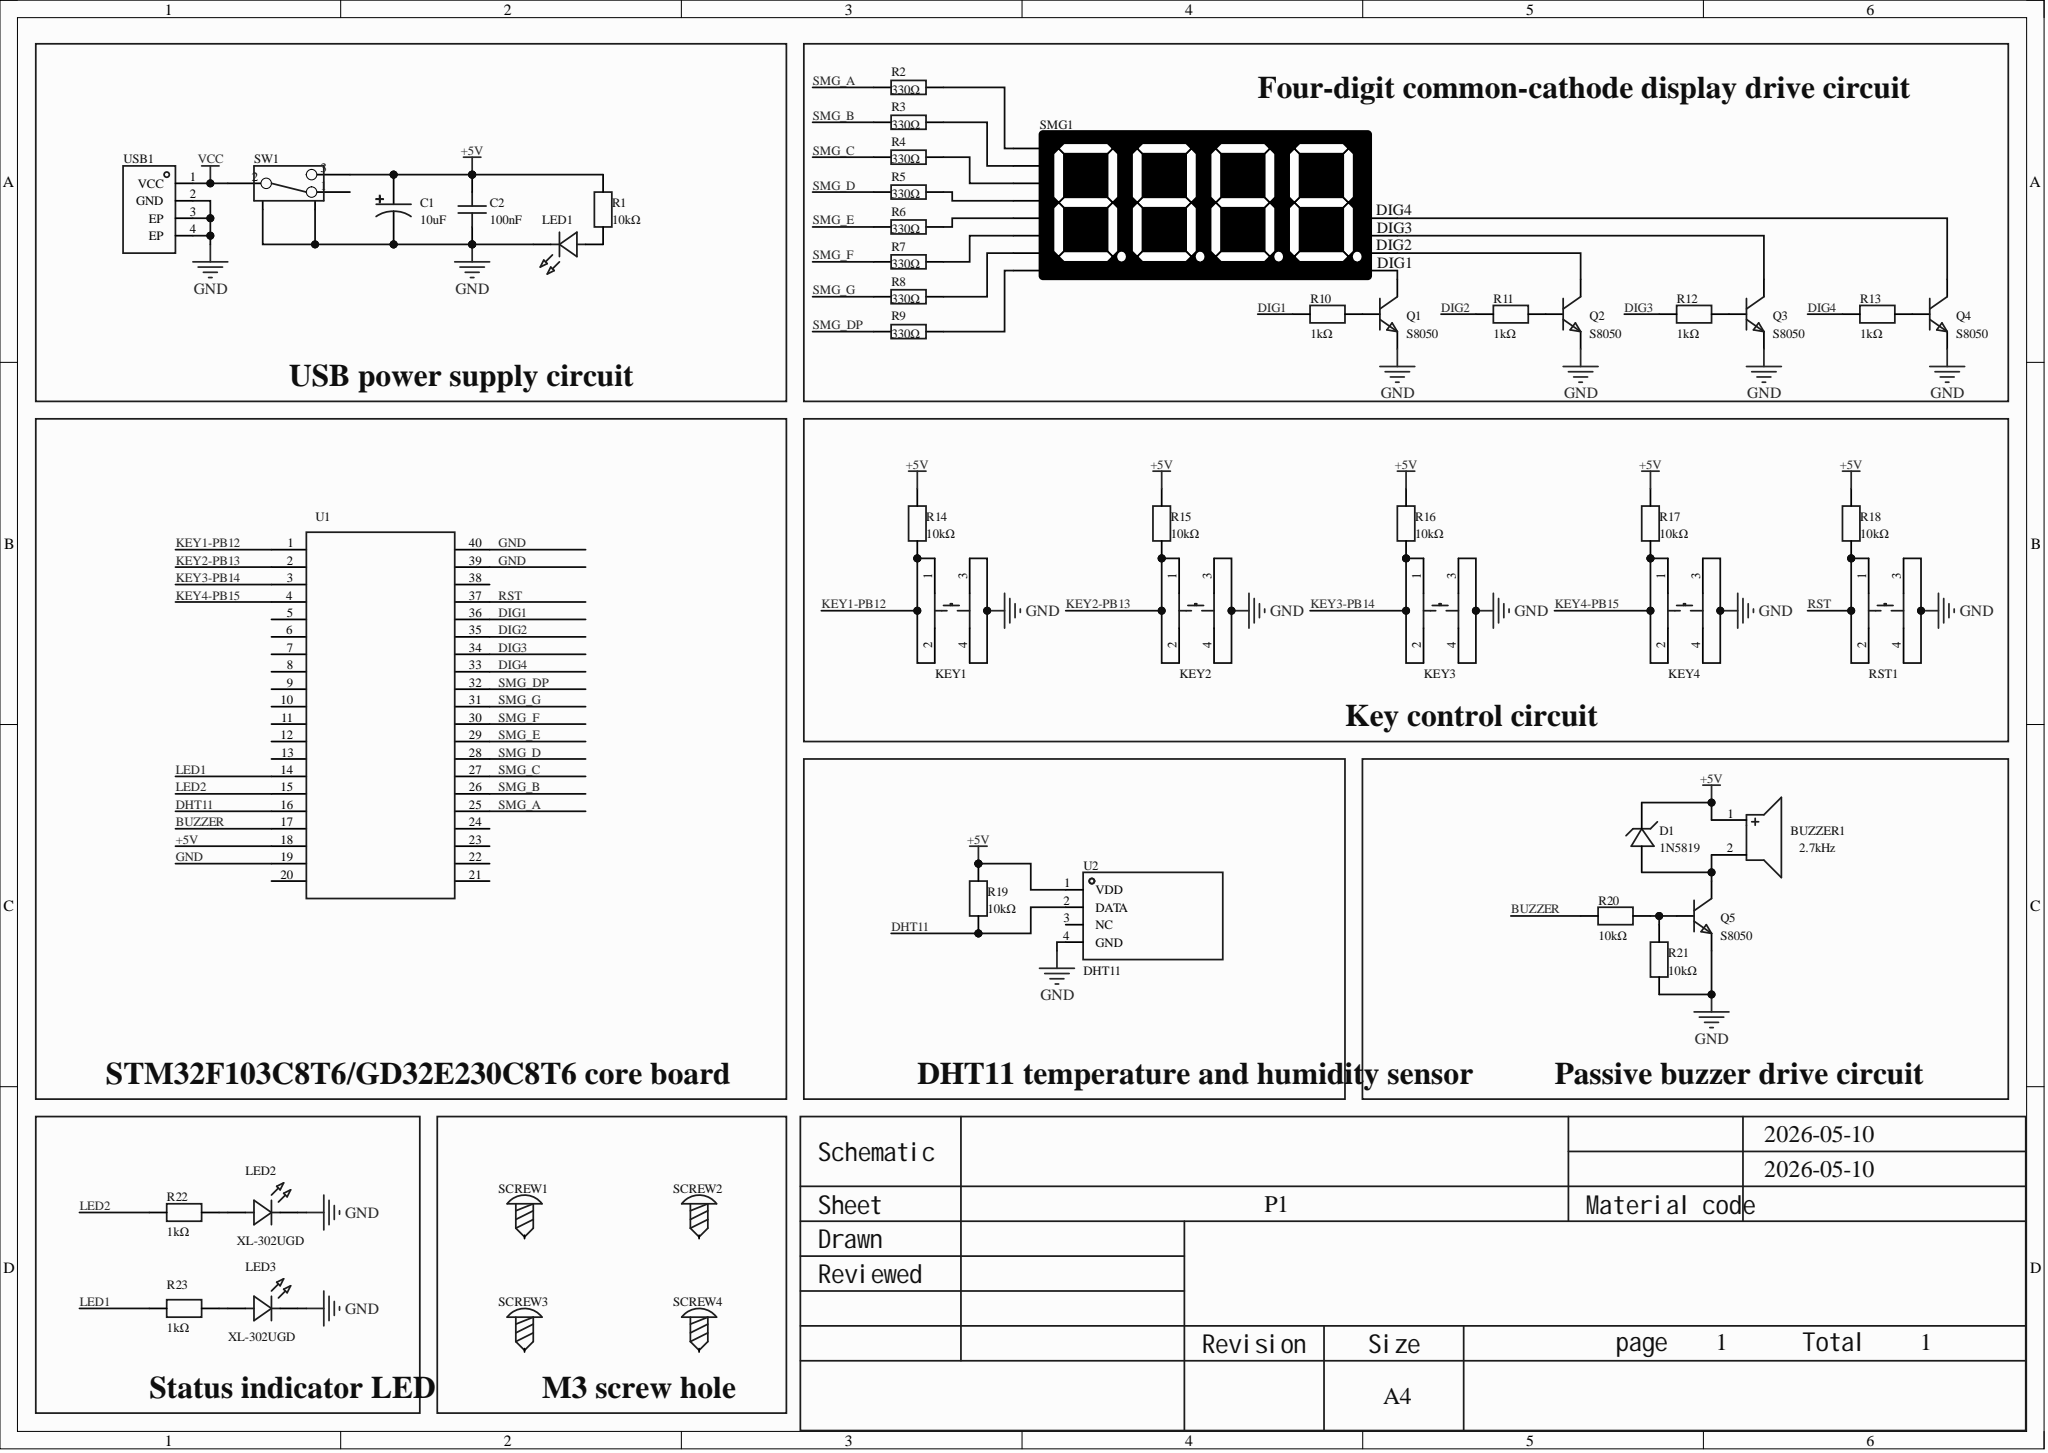Circuit board | Altium Designer | 49 parts | 45 nets
Bill of materials:
Comment,Description,Designator,Footprint,LibRef,Quantity
"2.7kHz","Drive mode: passive (external drive); construction: electromagnetic; frequency: 2.7kHz; sound pressure (SPL): 85dB@3V,10cm;","BUZZER1","BUZ-TH_BD9.0-P4.00-D0.6-FD","QMB-09B-03","1"
"10uF","Capacitance: 10uF; tolerance: ±20%; rated voltage: 25V;","C1","CAP-TH_BD4.0-P1.50-D0.8-FD","KF1E100MB050A00CV0","1"
"100nF","Capacitance: 100nF; tolerance: -20%~+80%; rated voltage: 50V; temperature coefficient: Y5V;","C2","CAP-TH_L5.0-W2.5-P5.08-D0.7","CC1H104ZC74D3F5O30MN","1"
"1N5819","Forward voltage drop (Vf): 900mV@3A; DC reverse withstand voltage (Vr): 40V; average rectified current (Io): 1A;","D1","DO-41_BD2.4-L4.7-P8.70-D0.9-RD","1N5819_C402218","1"
"TS-1002-07026","Circuit structure: single pole single throw; button shape: round button; mounting: through-hole; switch length: 6mm; switch width: 6mm; switch height: 7mm; contact current: 50mA; rated voltage (DC): 12V; with light: -; mechanical life: -;","KEY1, KEY2, KEY3, KEY4, RST1","SW-TH_4P-L6.0-W6.0-P4.50-LS6.5","TS-1002-07026","5"
"XL-302SURD","","LED1","LED-TH_BD3.8-P2.54-RD","XL-302SURD","1"
"XL-302UGD","","LED2, LED3","LED-TH_BD3.8-P2.54-FD_GREEN","XL-302UGD","2"
"S8050","Transistor type: NPN; collector current (Ic): 500mA; collector-emitter breakdown voltage (Vceo): 25V; power (Pd): 625mW; DC current gain (hFE@Ic,Vce): 160@50mA,1V;","Q1, Q2, Q3, Q4, Q5","TO-92-3_L4.5-W3.5-P1.27-L","S8050_C2931492","5"
"10kΩ","Resistor type: metal film resistor; resistance: 10kΩ; tolerance: ±5%; power: 250mW;","R1, R14, R15, R16, R17, R18, R19, R20, R21","RES-TH_BD2.4-L6.3-P10.30-D0.6","MFR-25JT-52-10K","9"
"330Ω","Resistor type: metal film resistor; resistance: 330Ω; tolerance: ±1%; power: 250mW; temperature coefficient: ±50ppm/?;","R2, R3, R4, R5, R6, R7, R8, R9","RES-TH_BD2.2-L6.5-P10.50-D0.6","MFR-25FTE52-330R","8"
"1kΩ","Resistor type: metal film resistor; resistance: 1kΩ; tolerance: ±5%; power: 250mW;","R10, R11, R12, R13, R22, R23","RES-TH_BD2.2-L6.5-P10.50-D0.6","MFR-25JT-52-1K","6"
"","","SCREW1, SCREW2, SCREW3, SCREW4","M3螺丝","M3螺丝","4"
"","","SMG1","LED-SEG-TH_FJ5461AH","LED_SEG_TH_0.56x4","1"
"SK-12E12-G5","Circuit structure: single pole double throw; mounting: side entry; rated current (DC): -; rated voltage (DC): -; rated current (AC): -; rated voltage (AC): -; mechanical life: 5 thousand cycles;","SW1","SW-TH_SK-12E12-G5","SK-12E12-G5","1"
"GD32E230C8T6 minimum system board","","U1","GD32E230C8T6最小系统","GD32E230C8T6最小系统板","1"
"DHT11","New capacitive digital temperature and humidity sensor; old version discontinued; 16.1x12.6x5.8mm","U2","SENSOR-TH_DHT11","DHT11","1"
"KH-TYPE-C-2P","Connector type: -; standard: -; male/female: -; number of contacts: -; number of ports: -; mounting: -; rated current - power: -; contact material: -; contact plating: -; operating temperature range: -;","USB1","USB-SMD_KH-TYPE-C-2P","KH-TYPE-C-2P","1"
Netlist (Protel format):
[
BUZZER1
BUZ-TH_BD9.0-P4.00-D0.6-FD
2.7kHz



]
[
C1
CAP-TH_BD4.0-P1.50-D0.8-FD
10uF



]
[
C2
CAP-TH_L5.0-W2.5-P5.08-D0.7
100nF



]
[
D1
DO-41_BD2.4-L4.7-P8.70-D0.9-RD
1N5819



]
[
KEY1
SW-TH_4P-L6.0-W6.0-P4.50-LS6.5
TS-1002-07026



]
[
KEY2
SW-TH_4P-L6.0-W6.0-P4.50-LS6.5
TS-1002-07026



]
[
KEY3
SW-TH_4P-L6.0-W6.0-P4.50-LS6.5
TS-1002-07026



]
[
KEY4
SW-TH_4P-L6.0-W6.0-P4.50-LS6.5
TS-1002-07026



]
[
LED1
LED-TH_BD3.8-P2.54-RD
XL-302SURD



]
[
LED2
LED-TH_BD3.8-P2.54-FD_GREEN
XL-302UGD



]
[
LED3
LED-TH_BD3.8-P2.54-FD_GREEN
XL-302UGD



]
[
Q1
TO-92-3_L4.5-W3.5-P1.27-L
S8050



]
[
Q2
TO-92-3_L4.5-W3.5-P1.27-L
S8050



]
[
Q3
TO-92-3_L4.5-W3.5-P1.27-L
S8050



]
[
Q4
TO-92-3_L4.5-W3.5-P1.27-L
S8050



]
[
Q5
TO-92-3_L4.5-W3.5-P1.27-L
S8050



]
[
R1
RES-TH_BD2.4-L6.3-P10.30-D0.6
10kΩ



]
[
R2
RES-TH_BD2.2-L6.5-P10.50-D0.6
330Ω



]
[
R3
RES-TH_BD2.2-L6.5-P10.50-D0.6
330Ω



]
[
R4
RES-TH_BD2.2-L6.5-P10.50-D0.6
330Ω



]
[
R5
RES-TH_BD2.2-L6.5-P10.50-D0.6
330Ω



]
[
R6
RES-TH_BD2.2-L6.5-P10.50-D0.6
330Ω



]
[
R7
RES-TH_BD2.2-L6.5-P10.50-D0.6
330Ω



]
[
R8
RES-TH_BD2.2-L6.5-P10.50-D0.6
330Ω



]
[
R9
RES-TH_BD2.2-L6.5-P10.50-D0.6
330Ω



]
[
R10
RES-TH_BD2.2-L6.5-P10.50-D0.6
1kΩ



]
[
R11
RES-TH_BD2.2-L6.5-P10.50-D0.6
1kΩ



]
[
R12
RES-TH_BD2.2-L6.5-P10.50-D0.6
1kΩ



]
[
R13
RES-TH_BD2.2-L6.5-P10.50-D0.6
1kΩ



]
[
R14
RES-TH_BD2.4-L6.3-P10.30-D0.6
10kΩ



]
[
R15
RES-TH_BD2.4-L6.3-P10.30-D0.6
10kΩ



]
[
R16
RES-TH_BD2.4-L6.3-P10.30-D0.6
10kΩ



]
[
R17
RES-TH_BD2.4-L6.3-P10.30-D0.6
10kΩ



]
[
R18
RES-TH_BD2.4-L6.3-P10.30-D0.6
10kΩ



]
[
R19
RES-TH_BD2.4-L6.3-P10.30-D0.6
10kΩ



]
[
R20
RES-TH_BD2.4-L6.3-P10.30-D0.6
10kΩ



]
[
R21
RES-TH_BD2.4-L6.3-P10.30-D0.6
10kΩ



]
[
R22
RES-TH_BD2.2-L6.5-P10.50-D0.6
1kΩ



]
[
R23
RES-TH_BD2.2-L6.5-P10.50-D0.6
1kΩ



]
[
RST1
SW-TH_4P-L6.0-W6.0-P4.50-LS6.5
TS-1002-07026



]
[
SCREW1
M3螺丝




]
[
SCREW2
M3螺丝




]
[
SCREW3
M3螺丝




]
[
SCREW4
M3螺丝




]
[
SMG1
LED-SEG-TH_FJ5461AH




]
[
SW1
SW-TH_SK-12E12-G5
SK-12E12-G5



]
[
U1
GD32E230C8T6最小系统
GD32E230C8T6 minimum system board



]
[
U2
SENSOR-TH_DHT11
DHT11



]
[
USB1
USB-SMD_KH-TYPE-C-2P
KH-TYPE-C-2P



]
(
VCC
SW1-2
USB1-1
)
(
SMG_G
R8-1
U1-31
)
(
SMG_F
R7-1
U1-30
)
(
SMG_E
R6-1
U1-29
)
(
SMG_DP
R9-1
U1-32
)
(
SMG_D
R5-1
U1-28
)
(
SMG_C
R4-1
U1-27
)
(
SMG_B
R3-1
U1-26
)
(
SMG_A
R2-1
U1-25
)
(
RST
R18-1
RST1-1
RST1-2
U1-37
)
(
NetR9_2
R9-2
SMG1-3
)
(
NetR8_2
R8-2
SMG1-5
)
(
NetR7_2
R7-2
SMG1-10
)
(
NetR6_2
R6-2
SMG1-1
)
(
NetR5_2
R5-2
SMG1-2
)
(
NetR4_2
R4-2
SMG1-4
)
(
NetR3_2
R3-2
SMG1-7
)
(
NetR2_2
R2-2
SMG1-11
)
(
NetQ5_2
Q5-2
R20-1
R21-2
)
(
NetQ4_3
Q4-3
SMG1-6
)
(
NetQ4_2
Q4-2
R13-1
)
(
NetQ3_3
Q3-3
SMG1-8
)
(
NetQ3_2
Q3-2
R12-1
)
(
NetQ2_3
Q2-3
SMG1-9
)
(
NetQ2_2
Q2-2
R11-1
)
(
NetQ1_3
Q1-3
SMG1-12
)
(
NetQ1_2
Q1-2
R10-1
)
(
NetLED3_1
LED3-1
R23-1
)
(
NetLED2_1
LED2-1
R22-1
)
(
NetLED1_2
LED1-2
R1-1
)
(
NetBUZZER1_2
BUZZER1-2
D1-2
Q5-3
)
(
LED2
R22-2
U1-15
)
(
LED1
R23-2
U1-14
)
(
KEY4-PB15
KEY4-1
KEY4-2
R17-1
U1-4
)
(
KEY3-PB14
KEY3-1
KEY3-2
R16-1
U1-3
)
(
KEY2-PB13
KEY2-1
KEY2-2
R15-1
U1-2
)
(
KEY1-PB12
KEY1-1
KEY1-2
R14-1
U1-1
)
(
GND
C1-2
C2-1
KEY1-3
KEY1-4
KEY2-3
KEY2-4
KEY3-3
KEY3-4
KEY4-3
KEY4-4
LED1-1
LED2-2
LED3-2
Q1-1
Q2-1
Q3-1
Q4-1
Q5-1
R21-1
RST1-3
RST1-4
SW1-4
SW1-5
U1-19
U1-39
U1-40
U2-4
USB1-2
USB1-3
USB1-4
)
(
DIG4
R13-2
U1-33
)
(
DIG3
R12-2
U1-34
)
(
DIG2
R11-2
U1-35
)
(
DIG1
R10-2
U1-36
)
(
DHT11
R19-1
U1-16
U2-2
)
(
BUZZER
R20-2
U1-17
)
(
+5V
BUZZER1-1
C1-1
C2-2
D1-1
R1-2
R14-2
R15-2
R16-2
R17-2
R18-2
R19-2
SW1-3
U1-18
U2-1
)